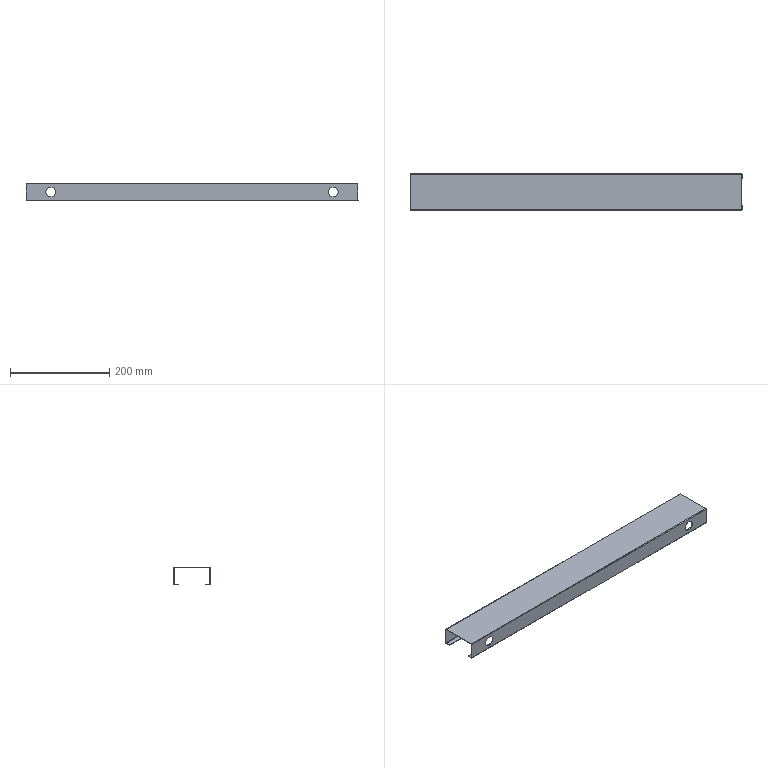Part | SolidWorks | features EdgeFlange 2, Cut 1, FlatPattern 1, ICE 1, SMBaseFlange 1, SheetMetal 1 | 1 solid | 46 faces | box 668 x 74 x 35 mm | volume 104821 mm3 | plane 30 | cylinder 16 | commonest cylinder face diameters 20 x8 0.4 x4 2.4 x4
STEP:
#1=CARTESIAN_POINT('',(-284.,36.,-27.5));
#2=VERTEX_POINT('',#1);
#3=CARTESIAN_POINT('',(-284.,36.,-7.5));
#4=VERTEX_POINT('',#3);
#5=CARTESIAN_POINT('',(-284.,36.,-17.5));
#6=DIRECTION('',(0.,1.,0.));
#7=DIRECTION('',(0.,0.,1.));
#8=AXIS2_PLACEMENT_3D('',#5,#6,#7);
#9=CIRCLE('',#8,10.);
#10=EDGE_CURVE('',#2,#4,#9,.T.);
#11=ORIENTED_EDGE('',*,*,#10,.F.);
#12=CARTESIAN_POINT('',(-284.,37.,-27.5));
#13=VERTEX_POINT('',#12);
#14=CARTESIAN_POINT('',(-284.,-37.,-27.5));
#15=DIRECTION('',(0.,1.,0.));
#16=VECTOR('',#15,1000.);
#17=LINE('',#14,#16);
#18=EDGE_CURVE('',#2,#13,#17,.T.);
#19=ORIENTED_EDGE('',*,*,#18,.T.);
#20=CARTESIAN_POINT('',(-284.,37.,-7.5));
#21=VERTEX_POINT('',#20);
#22=CARTESIAN_POINT('',(-284.,37.,-17.5));
#23=DIRECTION('',(0.,1.,0.));
#24=DIRECTION('',(0.,0.,1.));
#25=AXIS2_PLACEMENT_3D('',#22,#23,#24);
#26=CIRCLE('',#25,10.);
#27=EDGE_CURVE('',#13,#21,#26,.T.);
#28=ORIENTED_EDGE('',*,*,#27,.T.);
#29=CARTESIAN_POINT('',(-284.,-37.,-7.5));
#30=DIRECTION('',(0.,1.,0.));
#31=VECTOR('',#30,1000.);
#32=LINE('',#29,#31);
#33=EDGE_CURVE('',#4,#21,#32,.T.);
#34=ORIENTED_EDGE('',*,*,#33,.F.);
#35=EDGE_LOOP('',(#11,#19,#28,#34));
#36=FACE_OUTER_BOUND('',#35,.T.);
#37=CARTESIAN_POINT('',(-284.,-37.,-17.5));
#38=DIRECTION('',(0.,1.,0.));
#39=DIRECTION('',(0.,0.,1.));
#40=AXIS2_PLACEMENT_3D('',#37,#38,#39);
#41=CYLINDRICAL_SURFACE('',#40,10.);
#42=ADVANCED_FACE('',(#36),#41,.F.);
#43=CARTESIAN_POINT('',(284.,36.,-27.5));
#44=VERTEX_POINT('',#43);
#45=CARTESIAN_POINT('',(284.,36.,-7.5));
#46=VERTEX_POINT('',#45);
#47=CARTESIAN_POINT('',(284.,36.,-17.5));
#48=DIRECTION('',(0.,1.,0.));
#49=DIRECTION('',(0.,0.,1.));
#50=AXIS2_PLACEMENT_3D('',#47,#48,#49);
#51=CIRCLE('',#50,10.);
#52=EDGE_CURVE('',#44,#46,#51,.T.);
#53=ORIENTED_EDGE('',*,*,#52,.F.);
#54=CARTESIAN_POINT('',(284.,37.,-27.5));
#55=VERTEX_POINT('',#54);
#56=CARTESIAN_POINT('',(284.,-37.,-27.5));
#57=DIRECTION('',(0.,1.,0.));
#58=VECTOR('',#57,1000.);
#59=LINE('',#56,#58);
#60=EDGE_CURVE('',#44,#55,#59,.T.);
#61=ORIENTED_EDGE('',*,*,#60,.T.);
#62=CARTESIAN_POINT('',(284.,37.,-7.5));
#63=VERTEX_POINT('',#62);
#64=CARTESIAN_POINT('',(284.,37.,-17.5));
#65=DIRECTION('',(0.,1.,0.));
#66=DIRECTION('',(0.,0.,1.));
#67=AXIS2_PLACEMENT_3D('',#64,#65,#66);
#68=CIRCLE('',#67,10.);
#69=EDGE_CURVE('',#55,#63,#68,.T.);
#70=ORIENTED_EDGE('',*,*,#69,.T.);
#71=CARTESIAN_POINT('',(284.,-37.,-7.5));
#72=DIRECTION('',(0.,1.,0.));
#73=VECTOR('',#72,1000.);
#74=LINE('',#71,#73);
#75=EDGE_CURVE('',#46,#63,#74,.T.);
#76=ORIENTED_EDGE('',*,*,#75,.F.);
#77=EDGE_LOOP('',(#53,#61,#70,#76));
#78=FACE_OUTER_BOUND('',#77,.T.);
#79=CARTESIAN_POINT('',(284.,-37.,-17.5));
#80=DIRECTION('',(0.,1.,0.));
#81=DIRECTION('',(0.,0.,1.));
#82=AXIS2_PLACEMENT_3D('',#79,#80,#81);
#83=CYLINDRICAL_SURFACE('',#82,10.);
#84=ADVANCED_FACE('',(#78),#83,.F.);
#85=CARTESIAN_POINT('',(-284.,-37.,-27.5));
#86=VERTEX_POINT('',#85);
#87=CARTESIAN_POINT('',(-284.,-37.,-7.5));
#88=VERTEX_POINT('',#87);
#89=CARTESIAN_POINT('',(-284.,-37.,-17.5));
#90=DIRECTION('',(0.,1.,0.));
#91=DIRECTION('',(0.,0.,1.));
#92=AXIS2_PLACEMENT_3D('',#89,#90,#91);
#93=CIRCLE('',#92,10.);
#94=EDGE_CURVE('',#86,#88,#93,.T.);
#95=ORIENTED_EDGE('',*,*,#94,.F.);
#96=CARTESIAN_POINT('',(-284.,-36.,-27.5));
#97=VERTEX_POINT('',#96);
#98=CARTESIAN_POINT('',(-284.,-37.,-27.5));
#99=DIRECTION('',(0.,1.,0.));
#100=VECTOR('',#99,1000.);
#101=LINE('',#98,#100);
#102=EDGE_CURVE('',#86,#97,#101,.T.);
#103=ORIENTED_EDGE('',*,*,#102,.T.);
#104=CARTESIAN_POINT('',(-284.,-36.,-7.5));
#105=VERTEX_POINT('',#104);
#106=CARTESIAN_POINT('',(-284.,-36.,-17.5));
#107=DIRECTION('',(0.,1.,0.));
#108=DIRECTION('',(0.,0.,1.));
#109=AXIS2_PLACEMENT_3D('',#106,#107,#108);
#110=CIRCLE('',#109,10.);
#111=EDGE_CURVE('',#97,#105,#110,.T.);
#112=ORIENTED_EDGE('',*,*,#111,.T.);
#113=CARTESIAN_POINT('',(-284.,-37.,-7.5));
#114=DIRECTION('',(0.,1.,0.));
#115=VECTOR('',#114,1000.);
#116=LINE('',#113,#115);
#117=EDGE_CURVE('',#88,#105,#116,.T.);
#118=ORIENTED_EDGE('',*,*,#117,.F.);
#119=EDGE_LOOP('',(#95,#103,#112,#118));
#120=FACE_OUTER_BOUND('',#119,.T.);
#121=CARTESIAN_POINT('',(-284.,-37.,-17.5));
#122=DIRECTION('',(0.,1.,0.));
#123=DIRECTION('',(0.,0.,1.));
#124=AXIS2_PLACEMENT_3D('',#121,#122,#123);
#125=CYLINDRICAL_SURFACE('',#124,10.);
#126=ADVANCED_FACE('',(#120),#125,.F.);
#127=CARTESIAN_POINT('',(284.,-37.,-27.5));
#128=VERTEX_POINT('',#127);
#129=CARTESIAN_POINT('',(284.,-37.,-7.5));
#130=VERTEX_POINT('',#129);
#131=CARTESIAN_POINT('',(284.,-37.,-17.5));
#132=DIRECTION('',(0.,1.,0.));
#133=DIRECTION('',(0.,0.,-1.));
#134=AXIS2_PLACEMENT_3D('',#131,#132,#133);
#135=CIRCLE('',#134,10.);
#136=EDGE_CURVE('',#128,#130,#135,.T.);
#137=ORIENTED_EDGE('',*,*,#136,.F.);
#138=CARTESIAN_POINT('',(284.,-36.,-27.5));
#139=VERTEX_POINT('',#138);
#140=CARTESIAN_POINT('',(284.,-37.,-27.5));
#141=DIRECTION('',(0.,1.,0.));
#142=VECTOR('',#141,1000.);
#143=LINE('',#140,#142);
#144=EDGE_CURVE('',#128,#139,#143,.T.);
#145=ORIENTED_EDGE('',*,*,#144,.T.);
#146=CARTESIAN_POINT('',(284.,-36.,-7.5));
#147=VERTEX_POINT('',#146);
#148=CARTESIAN_POINT('',(284.,-36.,-17.5));
#149=DIRECTION('',(0.,1.,0.));
#150=DIRECTION('',(0.,0.,1.));
#151=AXIS2_PLACEMENT_3D('',#148,#149,#150);
#152=CIRCLE('',#151,10.);
#153=EDGE_CURVE('',#139,#147,#152,.T.);
#154=ORIENTED_EDGE('',*,*,#153,.T.);
#155=CARTESIAN_POINT('',(284.,-37.,-7.5));
#156=DIRECTION('',(0.,1.,0.));
#157=VECTOR('',#156,1000.);
#158=LINE('',#155,#157);
#159=EDGE_CURVE('',#130,#147,#158,.T.);
#160=ORIENTED_EDGE('',*,*,#159,.F.);
#161=EDGE_LOOP('',(#137,#145,#154,#160));
#162=FACE_OUTER_BOUND('',#161,.T.);
#163=CARTESIAN_POINT('',(284.,-37.,-17.5));
#164=DIRECTION('',(0.,1.,0.));
#165=DIRECTION('',(0.,0.,1.));
#166=AXIS2_PLACEMENT_3D('',#163,#164,#165);
#167=CYLINDRICAL_SURFACE('',#166,10.);
#168=ADVANCED_FACE('',(#162),#167,.F.);
#169=CARTESIAN_POINT('',(334.,36.,-33.8));
#170=VERTEX_POINT('',#169);
#171=CARTESIAN_POINT('',(334.,36.,-1.2));
#172=VERTEX_POINT('',#171);
#173=CARTESIAN_POINT('',(334.,36.,0.));
#174=DIRECTION('',(0.,0.,1.));
#175=VECTOR('',#174,1000.);
#176=LINE('',#173,#175);
#177=EDGE_CURVE('',#170,#172,#176,.T.);
#178=ORIENTED_EDGE('',*,*,#177,.F.);
#179=CARTESIAN_POINT('',(334.,37.,-33.8));
#180=VERTEX_POINT('',#179);
#181=CARTESIAN_POINT('',(334.,36.,-33.8));
#182=DIRECTION('',(0.,1.,0.));
#183=VECTOR('',#182,1000.);
#184=LINE('',#181,#183);
#185=EDGE_CURVE('',#170,#180,#184,.T.);
#186=ORIENTED_EDGE('',*,*,#185,.T.);
#187=CARTESIAN_POINT('',(334.,37.,-1.2));
#188=VERTEX_POINT('',#187);
#189=CARTESIAN_POINT('',(334.,37.,-1.));
#190=DIRECTION('',(0.,0.,1.));
#191=VECTOR('',#190,1000.);
#192=LINE('',#189,#191);
#193=EDGE_CURVE('',#180,#188,#192,.T.);
#194=ORIENTED_EDGE('',*,*,#193,.T.);
#195=CARTESIAN_POINT('',(334.,36.,-1.2));
#196=DIRECTION('',(0.,1.,0.));
#197=VECTOR('',#196,1000.);
#198=LINE('',#195,#197);
#199=EDGE_CURVE('',#172,#188,#198,.T.);
#200=ORIENTED_EDGE('',*,*,#199,.F.);
#201=EDGE_LOOP('',(#178,#186,#194,#200));
#202=FACE_OUTER_BOUND('',#201,.T.);
#203=CARTESIAN_POINT('',(334.,37.,-1.));
#204=DIRECTION('',(1.,0.,0.));
#205=DIRECTION('',(0.,0.,-1.));
#206=AXIS2_PLACEMENT_3D('',#203,#204,#205);
#207=PLANE('',#206);
#208=ADVANCED_FACE('',(#202),#207,.T.);
#209=CARTESIAN_POINT('',(-284.,37.,-17.5));
#210=DIRECTION('',(0.,1.,0.));
#211=DIRECTION('',(0.,0.,1.));
#212=AXIS2_PLACEMENT_3D('',#209,#210,#211);
#213=CIRCLE('',#212,10.);
#214=EDGE_CURVE('',#21,#13,#213,.T.);
#215=ORIENTED_EDGE('',*,*,#214,.F.);
#216=ORIENTED_EDGE('',*,*,#27,.F.);
#217=EDGE_LOOP('',(#215,#216));
#218=FACE_BOUND('',#217,.T.);
#219=CARTESIAN_POINT('',(284.,37.,-17.5));
#220=DIRECTION('',(0.,1.,0.));
#221=DIRECTION('',(0.,0.,1.));
#222=AXIS2_PLACEMENT_3D('',#219,#220,#221);
#223=CIRCLE('',#222,10.);
#224=EDGE_CURVE('',#63,#55,#223,.T.);
#225=ORIENTED_EDGE('',*,*,#224,.F.);
#226=ORIENTED_EDGE('',*,*,#69,.F.);
#227=EDGE_LOOP('',(#225,#226));
#228=FACE_BOUND('',#227,.T.);
#229=ORIENTED_EDGE('',*,*,#193,.F.);
#230=CARTESIAN_POINT('',(-334.,37.,-33.8));
#231=VERTEX_POINT('',#230);
#232=CARTESIAN_POINT('',(334.,37.,-33.8));
#233=DIRECTION('',(-1.,0.,0.));
#234=VECTOR('',#233,1000.);
#235=LINE('',#232,#234);
#236=EDGE_CURVE('',#180,#231,#235,.T.);
#237=ORIENTED_EDGE('',*,*,#236,.T.);
#238=CARTESIAN_POINT('',(-334.,37.,-1.2));
#239=VERTEX_POINT('',#238);
#240=CARTESIAN_POINT('',(-334.,37.,-35.));
#241=DIRECTION('',(0.,0.,-1.));
#242=VECTOR('',#241,1000.);
#243=LINE('',#240,#242);
#244=EDGE_CURVE('',#239,#231,#243,.T.);
#245=ORIENTED_EDGE('',*,*,#244,.F.);
#246=CARTESIAN_POINT('',(0.,37.,-1.2));
#247=DIRECTION('',(1.,0.,0.));
#248=VECTOR('',#247,1000.);
#249=LINE('',#246,#248);
#250=EDGE_CURVE('',#239,#188,#249,.T.);
#251=ORIENTED_EDGE('',*,*,#250,.T.);
#252=EDGE_LOOP('',(#229,#237,#245,#251));
#253=FACE_OUTER_BOUND('',#252,.T.);
#254=CARTESIAN_POINT('',(0.,37.,0.));
#255=DIRECTION('',(0.,1.,0.));
#256=DIRECTION('',(0.,0.,1.));
#257=AXIS2_PLACEMENT_3D('',#254,#255,#256);
#258=PLANE('',#257);
#259=ADVANCED_FACE('',(#218,#228,#253),#258,.T.);
#260=CARTESIAN_POINT('',(-284.,36.,-17.5));
#261=DIRECTION('',(0.,1.,0.));
#262=DIRECTION('',(0.,0.,1.));
#263=AXIS2_PLACEMENT_3D('',#260,#261,#262);
#264=CIRCLE('',#263,10.);
#265=EDGE_CURVE('',#4,#2,#264,.T.);
#266=ORIENTED_EDGE('',*,*,#265,.T.);
#267=ORIENTED_EDGE('',*,*,#10,.T.);
#268=EDGE_LOOP('',(#266,#267));
#269=FACE_BOUND('',#268,.T.);
#270=CARTESIAN_POINT('',(284.,36.,-17.5));
#271=DIRECTION('',(0.,1.,0.));
#272=DIRECTION('',(0.,0.,1.));
#273=AXIS2_PLACEMENT_3D('',#270,#271,#272);
#274=CIRCLE('',#273,10.);
#275=EDGE_CURVE('',#46,#44,#274,.T.);
#276=ORIENTED_EDGE('',*,*,#275,.T.);
#277=ORIENTED_EDGE('',*,*,#52,.T.);
#278=EDGE_LOOP('',(#276,#277));
#279=FACE_BOUND('',#278,.T.);
#280=CARTESIAN_POINT('',(-334.,36.,-33.8));
#281=VERTEX_POINT('',#280);
#282=CARTESIAN_POINT('',(334.,36.,-33.8));
#283=DIRECTION('',(-1.,0.,0.));
#284=VECTOR('',#283,1000.);
#285=LINE('',#282,#284);
#286=EDGE_CURVE('',#170,#281,#285,.T.);
#287=ORIENTED_EDGE('',*,*,#286,.F.);
#288=ORIENTED_EDGE('',*,*,#177,.T.);
#289=CARTESIAN_POINT('',(-334.,36.,-1.2));
#290=VERTEX_POINT('',#289);
#291=CARTESIAN_POINT('',(-334.,36.,-1.2));
#292=DIRECTION('',(1.,0.,0.));
#293=VECTOR('',#292,1000.);
#294=LINE('',#291,#293);
#295=EDGE_CURVE('',#290,#172,#294,.T.);
#296=ORIENTED_EDGE('',*,*,#295,.F.);
#297=CARTESIAN_POINT('',(-334.,36.,0.));
#298=DIRECTION('',(0.,0.,-1.));
#299=VECTOR('',#298,1000.);
#300=LINE('',#297,#299);
#301=EDGE_CURVE('',#290,#281,#300,.T.);
#302=ORIENTED_EDGE('',*,*,#301,.T.);
#303=EDGE_LOOP('',(#287,#288,#296,#302));
#304=FACE_OUTER_BOUND('',#303,.T.);
#305=CARTESIAN_POINT('',(0.,36.,0.));
#306=DIRECTION('',(0.,1.,0.));
#307=DIRECTION('',(0.,0.,1.));
#308=AXIS2_PLACEMENT_3D('',#305,#306,#307);
#309=PLANE('',#308);
#310=ADVANCED_FACE('',(#269,#279,#304),#309,.F.);
#311=CARTESIAN_POINT('',(-334.,-36.,-33.8));
#312=VERTEX_POINT('',#311);
#313=CARTESIAN_POINT('',(-334.,-36.,-1.2));
#314=VERTEX_POINT('',#313);
#315=CARTESIAN_POINT('',(-334.,-36.,0.));
#316=DIRECTION('',(0.,0.,1.));
#317=VECTOR('',#316,1000.);
#318=LINE('',#315,#317);
#319=EDGE_CURVE('',#312,#314,#318,.T.);
#320=ORIENTED_EDGE('',*,*,#319,.F.);
#321=CARTESIAN_POINT('',(-334.,-37.,-33.8));
#322=VERTEX_POINT('',#321);
#323=CARTESIAN_POINT('',(-334.,-36.,-33.8));
#324=DIRECTION('',(0.,-1.,0.));
#325=VECTOR('',#324,1000.);
#326=LINE('',#323,#325);
#327=EDGE_CURVE('',#312,#322,#326,.T.);
#328=ORIENTED_EDGE('',*,*,#327,.T.);
#329=CARTESIAN_POINT('',(-334.,-37.,-1.2));
#330=VERTEX_POINT('',#329);
#331=CARTESIAN_POINT('',(-334.,-37.,-35.));
#332=DIRECTION('',(0.,0.,1.));
#333=VECTOR('',#332,1000.);
#334=LINE('',#331,#333);
#335=EDGE_CURVE('',#322,#330,#334,.T.);
#336=ORIENTED_EDGE('',*,*,#335,.T.);
#337=CARTESIAN_POINT('',(-334.,-36.,-1.2));
#338=DIRECTION('',(0.,-1.,0.));
#339=VECTOR('',#338,1000.);
#340=LINE('',#337,#339);
#341=EDGE_CURVE('',#314,#330,#340,.T.);
#342=ORIENTED_EDGE('',*,*,#341,.F.);
#343=EDGE_LOOP('',(#320,#328,#336,#342));
#344=FACE_OUTER_BOUND('',#343,.T.);
#345=CARTESIAN_POINT('',(-334.,-37.,-35.));
#346=DIRECTION('',(-1.,0.,0.));
#347=DIRECTION('',(0.,0.,1.));
#348=AXIS2_PLACEMENT_3D('',#345,#346,#347);
#349=PLANE('',#348);
#350=ADVANCED_FACE('',(#344),#349,.T.);
#351=CARTESIAN_POINT('',(-284.,-37.,-17.5));
#352=DIRECTION('',(0.,1.,0.));
#353=DIRECTION('',(0.,0.,1.));
#354=AXIS2_PLACEMENT_3D('',#351,#352,#353);
#355=CIRCLE('',#354,10.);
#356=EDGE_CURVE('',#88,#86,#355,.T.);
#357=ORIENTED_EDGE('',*,*,#356,.T.);
#358=ORIENTED_EDGE('',*,*,#94,.T.);
#359=EDGE_LOOP('',(#357,#358));
#360=FACE_BOUND('',#359,.T.);
#361=CARTESIAN_POINT('',(284.,-37.,-17.5));
#362=DIRECTION('',(0.,1.,0.));
#363=DIRECTION('',(0.,0.,-1.));
#364=AXIS2_PLACEMENT_3D('',#361,#362,#363);
#365=CIRCLE('',#364,10.);
#366=EDGE_CURVE('',#130,#128,#365,.T.);
#367=ORIENTED_EDGE('',*,*,#366,.T.);
#368=ORIENTED_EDGE('',*,*,#136,.T.);
#369=EDGE_LOOP('',(#367,#368));
#370=FACE_BOUND('',#369,.T.);
#371=CARTESIAN_POINT('',(334.,-37.,-33.8));
#372=VERTEX_POINT('',#371);
#373=CARTESIAN_POINT('',(-334.,-37.,-33.8));
#374=DIRECTION('',(1.,0.,0.));
#375=VECTOR('',#374,1000.);
#376=LINE('',#373,#375);
#377=EDGE_CURVE('',#322,#372,#376,.T.);
#378=ORIENTED_EDGE('',*,*,#377,.T.);
#379=CARTESIAN_POINT('',(334.,-37.,-1.2));
#380=VERTEX_POINT('',#379);
#381=CARTESIAN_POINT('',(334.,-37.,-1.));
#382=DIRECTION('',(0.,0.,-1.));
#383=VECTOR('',#382,1000.);
#384=LINE('',#381,#383);
#385=EDGE_CURVE('',#380,#372,#384,.T.);
#386=ORIENTED_EDGE('',*,*,#385,.F.);
#387=CARTESIAN_POINT('',(334.,-37.,-1.2));
#388=DIRECTION('',(1.,0.,0.));
#389=VECTOR('',#388,1000.);
#390=LINE('',#387,#389);
#391=EDGE_CURVE('',#330,#380,#390,.T.);
#392=ORIENTED_EDGE('',*,*,#391,.F.);
#393=ORIENTED_EDGE('',*,*,#335,.F.);
#394=EDGE_LOOP('',(#378,#386,#392,#393));
#395=FACE_OUTER_BOUND('',#394,.T.);
#396=CARTESIAN_POINT('',(0.,-37.,0.));
#397=DIRECTION('',(0.,1.,0.));
#398=DIRECTION('',(0.,0.,1.));
#399=AXIS2_PLACEMENT_3D('',#396,#397,#398);
#400=PLANE('',#399);
#401=ADVANCED_FACE('',(#360,#370,#395),#400,.F.);
#402=CARTESIAN_POINT('',(-284.,-36.,-17.5));
#403=DIRECTION('',(0.,1.,0.));
#404=DIRECTION('',(0.,0.,1.));
#405=AXIS2_PLACEMENT_3D('',#402,#403,#404);
#406=CIRCLE('',#405,10.);
#407=EDGE_CURVE('',#105,#97,#406,.T.);
#408=ORIENTED_EDGE('',*,*,#407,.F.);
#409=ORIENTED_EDGE('',*,*,#111,.F.);
#410=EDGE_LOOP('',(#408,#409));
#411=FACE_BOUND('',#410,.T.);
#412=CARTESIAN_POINT('',(284.,-36.,-17.5));
#413=DIRECTION('',(0.,1.,0.));
#414=DIRECTION('',(0.,0.,1.));
#415=AXIS2_PLACEMENT_3D('',#412,#413,#414);
#416=CIRCLE('',#415,10.);
#417=EDGE_CURVE('',#147,#139,#416,.T.);
#418=ORIENTED_EDGE('',*,*,#417,.F.);
#419=ORIENTED_EDGE('',*,*,#153,.F.);
#420=EDGE_LOOP('',(#418,#419));
#421=FACE_BOUND('',#420,.T.);
#422=CARTESIAN_POINT('',(334.,-36.,-1.2));
#423=VERTEX_POINT('',#422);
#424=CARTESIAN_POINT('',(334.,-36.,-33.8));
#425=VERTEX_POINT('',#424);
#426=CARTESIAN_POINT('',(334.,-36.,0.));
#427=DIRECTION('',(0.,0.,-1.));
#428=VECTOR('',#427,1000.);
#429=LINE('',#426,#428);
#430=EDGE_CURVE('',#423,#425,#429,.T.);
#431=ORIENTED_EDGE('',*,*,#430,.T.);
#432=CARTESIAN_POINT('',(-334.,-36.,-33.8));
#433=DIRECTION('',(1.,0.,0.));
#434=VECTOR('',#433,1000.);
#435=LINE('',#432,#434);
#436=EDGE_CURVE('',#312,#425,#435,.T.);
#437=ORIENTED_EDGE('',*,*,#436,.F.);
#438=ORIENTED_EDGE('',*,*,#319,.T.);
#439=CARTESIAN_POINT('',(334.,-36.,-1.2));
#440=DIRECTION('',(-1.,0.,0.));
#441=VECTOR('',#440,1000.);
#442=LINE('',#439,#441);
#443=EDGE_CURVE('',#423,#314,#442,.T.);
#444=ORIENTED_EDGE('',*,*,#443,.F.);
#445=EDGE_LOOP('',(#431,#437,#438,#444));
#446=FACE_OUTER_BOUND('',#445,.T.);
#447=CARTESIAN_POINT('',(0.,-36.,0.));
#448=DIRECTION('',(0.,1.,0.));
#449=DIRECTION('',(0.,0.,1.));
#450=AXIS2_PLACEMENT_3D('',#447,#448,#449);
#451=PLANE('',#450);
#452=ADVANCED_FACE('',(#411,#421,#446),#451,.T.);
#453=CARTESIAN_POINT('',(-334.,-35.8,-1.));
#454=VERTEX_POINT('',#453);
#455=CARTESIAN_POINT('',(334.,-35.8,-1.));
#456=VERTEX_POINT('',#455);
#457=CARTESIAN_POINT('',(-334.,-35.8,-1.));
#458=DIRECTION('',(1.,0.,0.));
#459=VECTOR('',#458,1000.);
#460=LINE('',#457,#459);
#461=EDGE_CURVE('',#454,#456,#460,.T.);
#462=ORIENTED_EDGE('',*,*,#461,.F.);
#463=CARTESIAN_POINT('',(-334.,35.8,-1.));
#464=VERTEX_POINT('',#463);
#465=CARTESIAN_POINT('',(-334.,37.,-1.));
#466=DIRECTION('',(0.,-1.,0.));
#467=VECTOR('',#466,1000.);
#468=LINE('',#465,#467);
#469=EDGE_CURVE('',#464,#454,#468,.T.);
#470=ORIENTED_EDGE('',*,*,#469,.F.);
#471=CARTESIAN_POINT('',(334.,35.8,-1.));
#472=VERTEX_POINT('',#471);
#473=CARTESIAN_POINT('',(334.,35.8,-1.));
#474=DIRECTION('',(-1.,0.,0.));
#475=VECTOR('',#474,1000.);
#476=LINE('',#473,#475);
#477=EDGE_CURVE('',#472,#464,#476,.T.);
#478=ORIENTED_EDGE('',*,*,#477,.F.);
#479=CARTESIAN_POINT('',(334.,37.,-1.));
#480=DIRECTION('',(0.,1.,0.));
#481=VECTOR('',#480,1000.);
#482=LINE('',#479,#481);
#483=EDGE_CURVE('',#456,#472,#482,.T.);
#484=ORIENTED_EDGE('',*,*,#483,.F.);
#485=EDGE_LOOP('',(#462,#470,#478,#484));
#486=FACE_OUTER_BOUND('',#485,.T.);
#487=CARTESIAN_POINT('',(0.,0.,-1.));
#488=DIRECTION('',(0.,0.,1.));
#489=DIRECTION('',(1.,0.,0.));
#490=AXIS2_PLACEMENT_3D('',#487,#488,#489);
#491=PLANE('',#490);
#492=ADVANCED_FACE('',(#486),#491,.F.);
#493=CARTESIAN_POINT('',(-334.,35.8,0.));
#494=VERTEX_POINT('',#493);
#495=CARTESIAN_POINT('',(-334.,-35.8,0.));
#496=VERTEX_POINT('',#495);
#497=CARTESIAN_POINT('',(-334.,37.,0.));
#498=DIRECTION('',(0.,-1.,0.));
#499=VECTOR('',#498,1000.);
#500=LINE('',#497,#499);
#501=EDGE_CURVE('',#494,#496,#500,.T.);
#502=ORIENTED_EDGE('',*,*,#501,.T.);
#503=CARTESIAN_POINT('',(334.,-35.8,0.));
#504=VERTEX_POINT('',#503);
#505=CARTESIAN_POINT('',(-334.,-35.8,0.));
#506=DIRECTION('',(1.,0.,0.));
#507=VECTOR('',#506,1000.);
#508=LINE('',#505,#507);
#509=EDGE_CURVE('',#496,#504,#508,.T.);
#510=ORIENTED_EDGE('',*,*,#509,.T.);
#511=CARTESIAN_POINT('',(334.,35.8,0.));
#512=VERTEX_POINT('',#511);
#513=CARTESIAN_POINT('',(334.,37.,0.));
#514=DIRECTION('',(0.,1.,0.));
#515=VECTOR('',#514,1000.);
#516=LINE('',#513,#515);
#517=EDGE_CURVE('',#504,#512,#516,.T.);
#518=ORIENTED_EDGE('',*,*,#517,.T.);
#519=CARTESIAN_POINT('',(334.,35.8,0.));
#520=DIRECTION('',(-1.,0.,0.));
#521=VECTOR('',#520,1000.);
#522=LINE('',#519,#521);
#523=EDGE_CURVE('',#512,#494,#522,.T.);
#524=ORIENTED_EDGE('',*,*,#523,.T.);
#525=EDGE_LOOP('',(#502,#510,#518,#524));
#526=FACE_OUTER_BOUND('',#525,.T.);
#527=CARTESIAN_POINT('',(0.,0.,0.));
#528=DIRECTION('',(0.,0.,1.));
#529=DIRECTION('',(1.,0.,0.));
#530=AXIS2_PLACEMENT_3D('',#527,#528,#529);
#531=PLANE('',#530);
#532=ADVANCED_FACE('',(#526),#531,.T.);
#533=ORIENTED_EDGE('',*,*,#469,.T.);
#534=CARTESIAN_POINT('',(-334.,-35.8,-1.));
#535=DIRECTION('',(0.,0.,1.));
#536=VECTOR('',#535,1000.);
#537=LINE('',#534,#536);
#538=EDGE_CURVE('',#454,#496,#537,.T.);
#539=ORIENTED_EDGE('',*,*,#538,.T.);
#540=ORIENTED_EDGE('',*,*,#501,.F.);
#541=CARTESIAN_POINT('',(-334.,35.8,-1.));
#542=DIRECTION('',(0.,0.,1.));
#543=VECTOR('',#542,1000.);
#544=LINE('',#541,#543);
#545=EDGE_CURVE('',#464,#494,#544,.T.);
#546=ORIENTED_EDGE('',*,*,#545,.F.);
#547=EDGE_LOOP('',(#533,#539,#540,#546));
#548=FACE_OUTER_BOUND('',#547,.T.);
#549=CARTESIAN_POINT('',(-334.,37.,-1.));
#550=DIRECTION('',(-1.,0.,0.));
#551=DIRECTION('',(0.,0.,1.));
#552=AXIS2_PLACEMENT_3D('',#549,#550,#551);
#553=PLANE('',#552);
#554=ADVANCED_FACE('',(#548),#553,.T.);
#555=CARTESIAN_POINT('',(334.,-35.8,-1.));
#556=DIRECTION('',(0.,0.,1.));
#557=VECTOR('',#556,1000.);
#558=LINE('',#555,#557);
#559=EDGE_CURVE('',#456,#504,#558,.T.);
#560=ORIENTED_EDGE('',*,*,#559,.F.);
#561=ORIENTED_EDGE('',*,*,#483,.T.);
#562=CARTESIAN_POINT('',(334.,35.8,-1.));
#563=DIRECTION('',(0.,0.,1.));
#564=VECTOR('',#563,1000.);
#565=LINE('',#562,#564);
#566=EDGE_CURVE('',#472,#512,#565,.T.);
#567=ORIENTED_EDGE('',*,*,#566,.T.);
#568=ORIENTED_EDGE('',*,*,#517,.F.);
#569=EDGE_LOOP('',(#560,#561,#567,#568));
#570=FACE_OUTER_BOUND('',#569,.T.);
#571=CARTESIAN_POINT('',(334.,37.,-1.));
#572=DIRECTION('',(1.,0.,0.));
#573=DIRECTION('',(0.,0.,-1.));
#574=AXIS2_PLACEMENT_3D('',#571,#572,#573);
#575=PLANE('',#574);
#576=ADVANCED_FACE('',(#570),#575,.T.);
#577=CARTESIAN_POINT('',(-334.,37.,-1.2));
#578=DIRECTION('',(0.,1.,0.));
#579=VECTOR('',#578,1000.);
#580=LINE('',#577,#579);
#581=EDGE_CURVE('',#290,#239,#580,.T.);
#582=ORIENTED_EDGE('',*,*,#581,.F.);
#583=CARTESIAN_POINT('',(-334.,35.8,-1.2));
#584=DIRECTION('',(-1.,0.,0.));
#585=DIRECTION('',(0.,0.,-1.));
#586=AXIS2_PLACEMENT_3D('',#583,#584,#585);
#587=CIRCLE('',#586,0.2);
#588=EDGE_CURVE('',#464,#290,#587,.T.);
#589=ORIENTED_EDGE('',*,*,#588,.F.);
#590=ORIENTED_EDGE('',*,*,#545,.T.);
#591=CARTESIAN_POINT('',(-334.,35.8,-1.2));
#592=DIRECTION('',(-1.,0.,0.));
#593=DIRECTION('',(0.,0.,-1.));
#594=AXIS2_PLACEMENT_3D('',#591,#592,#593);
#595=CIRCLE('',#594,1.2);
#596=EDGE_CURVE('',#494,#239,#595,.T.);
#597=ORIENTED_EDGE('',*,*,#596,.T.);
#598=EDGE_LOOP('',(#582,#589,#590,#597));
#599=FACE_OUTER_BOUND('',#598,.T.);
#600=CARTESIAN_POINT('',(-334.,35.8,-1.2));
#601=DIRECTION('',(-1.,0.,0.));
#602=DIRECTION('',(0.,0.,1.));
#603=AXIS2_PLACEMENT_3D('',#600,#601,#602);
#604=PLANE('',#603);
#605=ADVANCED_FACE('',(#599),#604,.T.);
#606=CARTESIAN_POINT('',(334.,35.8,-1.2));
#607=DIRECTION('',(1.,0.,0.));
#608=DIRECTION('',(0.,0.,-1.));
#609=AXIS2_PLACEMENT_3D('',#606,#607,#608);
#610=CIRCLE('',#609,0.2);
#611=EDGE_CURVE('',#172,#472,#610,.T.);
#612=ORIENTED_EDGE('',*,*,#611,.F.);
#613=ORIENTED_EDGE('',*,*,#199,.T.);
#614=CARTESIAN_POINT('',(334.,35.8,-1.2));
#615=DIRECTION('',(1.,0.,0.));
#616=DIRECTION('',(0.,0.,-1.));
#617=AXIS2_PLACEMENT_3D('',#614,#615,#616);
#618=CIRCLE('',#617,1.2);
#619=EDGE_CURVE('',#188,#512,#618,.T.);
#620=ORIENTED_EDGE('',*,*,#619,.T.);
#621=ORIENTED_EDGE('',*,*,#566,.F.);
#622=EDGE_LOOP('',(#612,#613,#620,#621));
#623=FACE_OUTER_BOUND('',#622,.T.);
#624=CARTESIAN_POINT('',(334.,35.8,-1.2));
#625=DIRECTION('',(-1.,0.,0.));
#626=DIRECTION('',(0.,0.,1.));
#627=AXIS2_PLACEMENT_3D('',#624,#625,#626);
#628=PLANE('',#627);
#629=ADVANCED_FACE('',(#623),#628,.F.);
#630=ORIENTED_EDGE('',*,*,#523,.F.);
#631=ORIENTED_EDGE('',*,*,#619,.F.);
#632=ORIENTED_EDGE('',*,*,#250,.F.);
#633=ORIENTED_EDGE('',*,*,#596,.F.);
#634=EDGE_LOOP('',(#630,#631,#632,#633));
#635=FACE_OUTER_BOUND('',#634,.T.);
#636=CARTESIAN_POINT('',(334.,35.8,-1.2));
#637=DIRECTION('',(1.,0.,0.));
#638=DIRECTION('',(0.,1.,0.));
#639=AXIS2_PLACEMENT_3D('',#636,#637,#638);
#640=CYLINDRICAL_SURFACE('',#639,1.2);
#641=ADVANCED_FACE('',(#635),#640,.T.);
#642=ORIENTED_EDGE('',*,*,#477,.T.);
#643=ORIENTED_EDGE('',*,*,#588,.T.);
#644=ORIENTED_EDGE('',*,*,#295,.T.);
#645=ORIENTED_EDGE('',*,*,#611,.T.);
#646=EDGE_LOOP('',(#642,#643,#644,#645));
#647=FACE_OUTER_BOUND('',#646,.T.);
#648=CARTESIAN_POINT('',(334.,35.8,-1.2));
#649=DIRECTION('',(1.,0.,0.));
#650=DIRECTION('',(0.,1.,0.));
#651=AXIS2_PLACEMENT_3D('',#648,#649,#650);
#652=CYLINDRICAL_SURFACE('',#651,0.2);
#653=ADVANCED_FACE('',(#647),#652,.F.);
#654=CARTESIAN_POINT('',(-334.,36.,-33.8));
#655=DIRECTION('',(0.,1.,0.));
#656=VECTOR('',#655,1000.);
#657=LINE('',#654,#656);
#658=EDGE_CURVE('',#281,#231,#657,.T.);
#659=ORIENTED_EDGE('',*,*,#658,.F.);
#660=ORIENTED_EDGE('',*,*,#301,.F.);
#661=ORIENTED_EDGE('',*,*,#581,.T.);
#662=ORIENTED_EDGE('',*,*,#244,.T.);
#663=EDGE_LOOP('',(#659,#660,#661,#662));
#664=FACE_OUTER_BOUND('',#663,.T.);
#665=CARTESIAN_POINT('',(-334.,37.,-35.));
#666=DIRECTION('',(-1.,0.,0.));
#667=DIRECTION('',(0.,0.,1.));
#668=AXIS2_PLACEMENT_3D('',#665,#666,#667);
#669=PLANE('',#668);
#670=ADVANCED_FACE('',(#664),#669,.T.);
#671=CARTESIAN_POINT('',(334.,-37.,-1.2));
#672=DIRECTION('',(0.,-1.,0.));
#673=VECTOR('',#672,1000.);
#674=LINE('',#671,#673);
#675=EDGE_CURVE('',#423,#380,#674,.T.);
#676=ORIENTED_EDGE('',*,*,#675,.F.);
#677=CARTESIAN_POINT('',(334.,-35.8,-1.2));
#678=DIRECTION('',(1.,0.,0.));
#679=DIRECTION('',(0.,0.,1.));
#680=AXIS2_PLACEMENT_3D('',#677,#678,#679);
#681=CIRCLE('',#680,0.2);
#682=EDGE_CURVE('',#456,#423,#681,.T.);
#683=ORIENTED_EDGE('',*,*,#682,.F.);
#684=ORIENTED_EDGE('',*,*,#559,.T.);
#685=CARTESIAN_POINT('',(334.,-35.8,-1.2));
#686=DIRECTION('',(1.,0.,0.));
#687=DIRECTION('',(0.,0.,1.));
#688=AXIS2_PLACEMENT_3D('',#685,#686,#687);
#689=CIRCLE('',#688,1.2);
#690=EDGE_CURVE('',#504,#380,#689,.T.);
#691=ORIENTED_EDGE('',*,*,#690,.T.);
#692=EDGE_LOOP('',(#676,#683,#684,#691));
#693=FACE_OUTER_BOUND('',#692,.T.);
#694=CARTESIAN_POINT('',(334.,-35.8,-1.2));
#695=DIRECTION('',(1.,0.,0.));
#696=DIRECTION('',(0.,0.,-1.));
#697=AXIS2_PLACEMENT_3D('',#694,#695,#696);
#698=PLANE('',#697);
#699=ADVANCED_FACE('',(#693),#698,.T.);
#700=CARTESIAN_POINT('',(-334.,-35.8,-1.2));
#701=DIRECTION('',(-1.,0.,0.));
#702=DIRECTION('',(0.,0.,1.));
#703=AXIS2_PLACEMENT_3D('',#700,#701,#702);
#704=CIRCLE('',#703,0.2);
#705=EDGE_CURVE('',#314,#454,#704,.T.);
#706=ORIENTED_EDGE('',*,*,#705,.F.);
#707=ORIENTED_EDGE('',*,*,#341,.T.);
#708=CARTESIAN_POINT('',(-334.,-35.8,-1.2));
#709=DIRECTION('',(-1.,0.,0.));
#710=DIRECTION('',(0.,0.,1.));
#711=AXIS2_PLACEMENT_3D('',#708,#709,#710);
#712=CIRCLE('',#711,1.2);
#713=EDGE_CURVE('',#330,#496,#712,.T.);
#714=ORIENTED_EDGE('',*,*,#713,.T.);
#715=ORIENTED_EDGE('',*,*,#538,.F.);
#716=EDGE_LOOP('',(#706,#707,#714,#715));
#717=FACE_OUTER_BOUND('',#716,.T.);
#718=CARTESIAN_POINT('',(-334.,-35.8,-1.2));
#719=DIRECTION('',(1.,0.,0.));
#720=DIRECTION('',(0.,0.,-1.));
#721=AXIS2_PLACEMENT_3D('',#718,#719,#720);
#722=PLANE('',#721);
#723=ADVANCED_FACE('',(#717),#722,.F.);
#724=ORIENTED_EDGE('',*,*,#509,.F.);
#725=ORIENTED_EDGE('',*,*,#713,.F.);
#726=ORIENTED_EDGE('',*,*,#391,.T.);
#727=ORIENTED_EDGE('',*,*,#690,.F.);
#728=EDGE_LOOP('',(#724,#725,#726,#727));
#729=FACE_OUTER_BOUND('',#728,.T.);
#730=CARTESIAN_POINT('',(-334.,-35.8,-1.2));
#731=DIRECTION('',(-1.,0.,0.));
#732=DIRECTION('',(0.,-1.,0.));
#733=AXIS2_PLACEMENT_3D('',#730,#731,#732);
#734=CYLINDRICAL_SURFACE('',#733,1.2);
#735=ADVANCED_FACE('',(#729),#734,.T.);
#736=ORIENTED_EDGE('',*,*,#461,.T.);
#737=ORIENTED_EDGE('',*,*,#682,.T.);
#738=ORIENTED_EDGE('',*,*,#443,.T.);
#739=ORIENTED_EDGE('',*,*,#705,.T.);
#740=EDGE_LOOP('',(#736,#737,#738,#739));
#741=FACE_OUTER_BOUND('',#740,.T.);
#742=CARTESIAN_POINT('',(-334.,-35.8,-1.2));
#743=DIRECTION('',(-1.,0.,0.));
#744=DIRECTION('',(0.,-1.,0.));
#745=AXIS2_PLACEMENT_3D('',#742,#743,#744);
#746=CYLINDRICAL_SURFACE('',#745,0.2);
#747=ADVANCED_FACE('',(#741),#746,.F.);
#748=CARTESIAN_POINT('',(334.,-36.,-33.8));
#749=DIRECTION('',(0.,-1.,0.));
#750=VECTOR('',#749,1000.);
#751=LINE('',#748,#750);
#752=EDGE_CURVE('',#425,#372,#751,.T.);
#753=ORIENTED_EDGE('',*,*,#752,.F.);
#754=ORIENTED_EDGE('',*,*,#430,.F.);
#755=ORIENTED_EDGE('',*,*,#675,.T.);
#756=ORIENTED_EDGE('',*,*,#385,.T.);
#757=EDGE_LOOP('',(#753,#754,#755,#756));
#758=FACE_OUTER_BOUND('',#757,.T.);
#759=CARTESIAN_POINT('',(334.,-37.,-1.));
#760=DIRECTION('',(1.,0.,0.));
#761=DIRECTION('',(0.,0.,-1.));
#762=AXIS2_PLACEMENT_3D('',#759,#760,#761);
#763=PLANE('',#762);
#764=ADVANCED_FACE('',(#758),#763,.T.);
#765=CARTESIAN_POINT('',(334.,-35.8,-34.));
#766=VERTEX_POINT('',#765);
#767=CARTESIAN_POINT('',(334.,-35.8,-35.));
#768=VERTEX_POINT('',#767);
#769=CARTESIAN_POINT('',(334.,-35.8,-35.));
#770=DIRECTION('',(0.,0.,-1.));
#771=VECTOR('',#770,1000.);
#772=LINE('',#769,#771);
#773=EDGE_CURVE('',#766,#768,#772,.T.);
#774=ORIENTED_EDGE('',*,*,#773,.F.);
#775=CARTESIAN_POINT('',(334.,-35.8,-33.8));
#776=DIRECTION('',(1.,0.,0.));
#777=DIRECTION('',(0.,0.,1.));
#778=AXIS2_PLACEMENT_3D('',#775,#776,#777);
#779=CIRCLE('',#778,0.2);
#780=EDGE_CURVE('',#425,#766,#779,.T.);
#781=ORIENTED_EDGE('',*,*,#780,.F.);
#782=ORIENTED_EDGE('',*,*,#752,.T.);
#783=CARTESIAN_POINT('',(334.,-35.8,-33.8));
#784=DIRECTION('',(1.,0.,0.));
#785=DIRECTION('',(0.,0.,1.));
#786=AXIS2_PLACEMENT_3D('',#783,#784,#785);
#787=CIRCLE('',#786,1.2);
#788=EDGE_CURVE('',#372,#768,#787,.T.);
#789=ORIENTED_EDGE('',*,*,#788,.T.);
#790=EDGE_LOOP('',(#774,#781,#782,#789));
#791=FACE_OUTER_BOUND('',#790,.T.);
#792=CARTESIAN_POINT('',(334.,-35.8,-33.8));
#793=DIRECTION('',(1.,0.,0.));
#794=DIRECTION('',(0.,0.,-1.));
#795=AXIS2_PLACEMENT_3D('',#792,#793,#794);
#796=PLANE('',#795);
#797=ADVANCED_FACE('',(#791),#796,.T.);
#798=CARTESIAN_POINT('',(-334.,-35.8,-34.));
#799=VERTEX_POINT('',#798);
#800=CARTESIAN_POINT('',(-334.,-35.8,-33.8));
#801=DIRECTION('',(-1.,0.,0.));
#802=DIRECTION('',(0.,0.,1.));
#803=AXIS2_PLACEMENT_3D('',#800,#801,#802);
#804=CIRCLE('',#803,0.2);
#805=EDGE_CURVE('',#799,#312,#804,.T.);
#806=ORIENTED_EDGE('',*,*,#805,.F.);
#807=CARTESIAN_POINT('',(-334.,-35.8,-35.));
#808=VERTEX_POINT('',#807);
#809=CARTESIAN_POINT('',(-334.,-35.8,-34.));
#810=DIRECTION('',(0.,0.,-1.));
#811=VECTOR('',#810,1000.);
#812=LINE('',#809,#811);
#813=EDGE_CURVE('',#799,#808,#812,.T.);
#814=ORIENTED_EDGE('',*,*,#813,.T.);
#815=CARTESIAN_POINT('',(-334.,-35.8,-33.8));
#816=DIRECTION('',(-1.,0.,0.));
#817=DIRECTION('',(0.,0.,1.));
#818=AXIS2_PLACEMENT_3D('',#815,#816,#817);
#819=CIRCLE('',#818,1.2);
#820=EDGE_CURVE('',#808,#322,#819,.T.);
#821=ORIENTED_EDGE('',*,*,#820,.T.);
#822=ORIENTED_EDGE('',*,*,#327,.F.);
#823=EDGE_LOOP('',(#806,#814,#821,#822));
#824=FACE_OUTER_BOUND('',#823,.T.);
#825=CARTESIAN_POINT('',(-334.,-35.8,-33.8));
#826=DIRECTION('',(1.,0.,0.));
#827=DIRECTION('',(0.,0.,-1.));
#828=AXIS2_PLACEMENT_3D('',#825,#826,#827);
#829=PLANE('',#828);
#830=ADVANCED_FACE('',(#824),#829,.F.);
#831=ORIENTED_EDGE('',*,*,#377,.F.);
#832=ORIENTED_EDGE('',*,*,#820,.F.);
#833=CARTESIAN_POINT('',(334.,-35.8,-35.));
#834=DIRECTION('',(1.,0.,0.));
#835=VECTOR('',#834,1000.);
#836=LINE('',#833,#835);
#837=EDGE_CURVE('',#808,#768,#836,.T.);
#838=ORIENTED_EDGE('',*,*,#837,.T.);
#839=ORIENTED_EDGE('',*,*,#788,.F.);
#840=EDGE_LOOP('',(#831,#832,#838,#839));
#841=FACE_OUTER_BOUND('',#840,.T.);
#842=CARTESIAN_POINT('',(-334.,-35.8,-33.8));
#843=DIRECTION('',(-1.,0.,0.));
#844=DIRECTION('',(0.,0.,-1.));
#845=AXIS2_PLACEMENT_3D('',#842,#843,#844);
#846=CYLINDRICAL_SURFACE('',#845,1.2);
#847=ADVANCED_FACE('',(#841),#846,.T.);
#848=ORIENTED_EDGE('',*,*,#436,.T.);
#849=ORIENTED_EDGE('',*,*,#780,.T.);
#850=CARTESIAN_POINT('',(334.,-35.8,-34.));
#851=DIRECTION('',(-1.,0.,0.));
#852=VECTOR('',#851,1000.);
#853=LINE('',#850,#852);
#854=EDGE_CURVE('',#766,#799,#853,.T.);
#855=ORIENTED_EDGE('',*,*,#854,.T.);
#856=ORIENTED_EDGE('',*,*,#805,.T.);
#857=EDGE_LOOP('',(#848,#849,#855,#856));
#858=FACE_OUTER_BOUND('',#857,.T.);
#859=CARTESIAN_POINT('',(-334.,-35.8,-33.8));
#860=DIRECTION('',(-1.,0.,0.));
#861=DIRECTION('',(0.,0.,-1.));
#862=AXIS2_PLACEMENT_3D('',#859,#860,#861);
#863=CYLINDRICAL_SURFACE('',#862,0.2);
#864=ADVANCED_FACE('',(#858),#863,.F.);
#865=ORIENTED_EDGE('',*,*,#773,.T.);
#866=CARTESIAN_POINT('',(334.,-27.,-35.));
#867=VERTEX_POINT('',#866);
#868=CARTESIAN_POINT('',(334.,0.,-35.));
#869=DIRECTION('',(0.,-1.,0.));
#870=VECTOR('',#869,1000.);
#871=LINE('',#868,#870);
#872=EDGE_CURVE('',#867,#768,#871,.T.);
#873=ORIENTED_EDGE('',*,*,#872,.F.);
#874=CARTESIAN_POINT('',(334.,-27.,-34.));
#875=VERTEX_POINT('',#874);
#876=CARTESIAN_POINT('',(334.,-27.,-35.));
#877=DIRECTION('',(0.,0.,1.));
#878=VECTOR('',#877,1000.);
#879=LINE('',#876,#878);
#880=EDGE_CURVE('',#867,#875,#879,.T.);
#881=ORIENTED_EDGE('',*,*,#880,.T.);
#882=CARTESIAN_POINT('',(334.,-36.,-34.));
#883=DIRECTION('',(0.,-1.,0.));
#884=VECTOR('',#883,1000.);
#885=LINE('',#882,#884);
#886=EDGE_CURVE('',#875,#766,#885,.T.);
#887=ORIENTED_EDGE('',*,*,#886,.T.);
#888=EDGE_LOOP('',(#865,#873,#881,#887));
#889=FACE_OUTER_BOUND('',#888,.T.);
#890=CARTESIAN_POINT('',(334.,-36.,-35.));
#891=DIRECTION('',(-1.,0.,0.));
#892=DIRECTION('',(0.,0.,1.));
#893=AXIS2_PLACEMENT_3D('',#890,#891,#892);
#894=PLANE('',#893);
#895=ADVANCED_FACE('',(#889),#894,.F.);
#896=ORIENTED_EDGE('',*,*,#813,.F.);
#897=CARTESIAN_POINT('',(-334.,-27.,-34.));
#898=VERTEX_POINT('',#897);
#899=CARTESIAN_POINT('',(-334.,-27.,-34.));
#900=DIRECTION('',(0.,1.,0.));
#901=VECTOR('',#900,1000.);
#902=LINE('',#899,#901);
#903=EDGE_CURVE('',#799,#898,#902,.T.);
#904=ORIENTED_EDGE('',*,*,#903,.T.);
#905=CARTESIAN_POINT('',(-334.,-27.,-35.));
#906=VERTEX_POINT('',#905);
#907=CARTESIAN_POINT('',(-334.,-27.,-35.));
#908=DIRECTION('',(0.,0.,1.));
#909=VECTOR('',#908,1000.);
#910=LINE('',#907,#909);
#911=EDGE_CURVE('',#906,#898,#910,.T.);
#912=ORIENTED_EDGE('',*,*,#911,.F.);
#913=CARTESIAN_POINT('',(-334.,0.,-35.));
#914=DIRECTION('',(0.,1.,0.));
#915=VECTOR('',#914,1000.);
#916=LINE('',#913,#915);
#917=EDGE_CURVE('',#808,#906,#916,.T.);
#918=ORIENTED_EDGE('',*,*,#917,.F.);
#919=EDGE_LOOP('',(#896,#904,#912,#918));
#920=FACE_OUTER_BOUND('',#919,.T.);
#921=CARTESIAN_POINT('',(-334.,-27.,-35.));
#922=DIRECTION('',(1.,0.,0.));
#923=DIRECTION('',(0.,0.,-1.));
#924=AXIS2_PLACEMENT_3D('',#921,#922,#923);
#925=PLANE('',#924);
#926=ADVANCED_FACE('',(#920),#925,.F.);
#927=ORIENTED_EDGE('',*,*,#837,.F.);
#928=ORIENTED_EDGE('',*,*,#917,.T.);
#929=CARTESIAN_POINT('',(0.,-27.,-35.));
#930=DIRECTION('',(1.,0.,0.));
#931=VECTOR('',#930,1000.);
#932=LINE('',#929,#931);
#933=EDGE_CURVE('',#906,#867,#932,.T.);
#934=ORIENTED_EDGE('',*,*,#933,.T.);
#935=ORIENTED_EDGE('',*,*,#872,.T.);
#936=EDGE_LOOP('',(#927,#928,#934,#935));
#937=FACE_OUTER_BOUND('',#936,.T.);
#938=CARTESIAN_POINT('',(0.,0.,-35.));
#939=DIRECTION('',(0.,0.,1.));
#940=DIRECTION('',(0.,-1.,0.));
#941=AXIS2_PLACEMENT_3D('',#938,#939,#940);
#942=PLANE('',#941);
#943=ADVANCED_FACE('',(#937),#942,.F.);
#944=ORIENTED_EDGE('',*,*,#903,.F.);
#945=ORIENTED_EDGE('',*,*,#854,.F.);
#946=ORIENTED_EDGE('',*,*,#886,.F.);
#947=CARTESIAN_POINT('',(334.,-27.,-34.));
#948=DIRECTION('',(1.,0.,0.));
#949=VECTOR('',#948,1000.);
#950=LINE('',#947,#949);
#951=EDGE_CURVE('',#898,#875,#950,.T.);
#952=ORIENTED_EDGE('',*,*,#951,.F.);
#953=EDGE_LOOP('',(#944,#945,#946,#952));
#954=FACE_OUTER_BOUND('',#953,.T.);
#955=CARTESIAN_POINT('',(0.,0.,-34.));
#956=DIRECTION('',(0.,0.,1.));
#957=DIRECTION('',(0.,-1.,0.));
#958=AXIS2_PLACEMENT_3D('',#955,#956,#957);
#959=PLANE('',#958);
#960=ADVANCED_FACE('',(#954),#959,.T.);
#961=ORIENTED_EDGE('',*,*,#951,.T.);
#962=ORIENTED_EDGE('',*,*,#880,.F.);
#963=ORIENTED_EDGE('',*,*,#933,.F.);
#964=ORIENTED_EDGE('',*,*,#911,.T.);
#965=EDGE_LOOP('',(#961,#962,#963,#964));
#966=FACE_OUTER_BOUND('',#965,.T.);
#967=CARTESIAN_POINT('',(334.,-27.,-35.));
#968=DIRECTION('',(0.,-1.,0.));
#969=DIRECTION('',(0.,0.,-1.));
#970=AXIS2_PLACEMENT_3D('',#967,#968,#969);
#971=PLANE('',#970);
#972=ADVANCED_FACE('',(#966),#971,.F.);
#973=CARTESIAN_POINT('',(-334.,35.8,-34.));
#974=VERTEX_POINT('',#973);
#975=CARTESIAN_POINT('',(-334.,35.8,-35.));
#976=VERTEX_POINT('',#975);
#977=CARTESIAN_POINT('',(-334.,35.8,-35.));
#978=DIRECTION('',(0.,0.,-1.));
#979=VECTOR('',#978,1000.);
#980=LINE('',#977,#979);
#981=EDGE_CURVE('',#974,#976,#980,.T.);
#982=ORIENTED_EDGE('',*,*,#981,.F.);
#983=CARTESIAN_POINT('',(-334.,35.8,-33.8));
#984=DIRECTION('',(-1.,0.,0.));
#985=DIRECTION('',(0.,0.,-1.));
#986=AXIS2_PLACEMENT_3D('',#983,#984,#985);
#987=CIRCLE('',#986,0.2);
#988=EDGE_CURVE('',#281,#974,#987,.T.);
#989=ORIENTED_EDGE('',*,*,#988,.F.);
#990=ORIENTED_EDGE('',*,*,#658,.T.);
#991=CARTESIAN_POINT('',(-334.,35.8,-33.8));
#992=DIRECTION('',(-1.,0.,0.));
#993=DIRECTION('',(0.,0.,-1.));
#994=AXIS2_PLACEMENT_3D('',#991,#992,#993);
#995=CIRCLE('',#994,1.2);
#996=EDGE_CURVE('',#231,#976,#995,.T.);
#997=ORIENTED_EDGE('',*,*,#996,.T.);
#998=EDGE_LOOP('',(#982,#989,#990,#997));
#999=FACE_OUTER_BOUND('',#998,.T.);
#1000=CARTESIAN_POINT('',(-334.,35.8,-33.8));
#1001=DIRECTION('',(-1.,0.,0.));
#1002=DIRECTION('',(0.,0.,1.));
#1003=AXIS2_PLACEMENT_3D('',#1000,#1001,#1002);
#1004=PLANE('',#1003);
#1005=ADVANCED_FACE('',(#999),#1004,.T.);
#1006=CARTESIAN_POINT('',(334.,35.8,-34.));
#1007=VERTEX_POINT('',#1006);
#1008=CARTESIAN_POINT('',(334.,35.8,-33.8));
#1009=DIRECTION('',(1.,0.,0.));
#1010=DIRECTION('',(0.,0.,-1.));
#1011=AXIS2_PLACEMENT_3D('',#1008,#1009,#1010);
#1012=CIRCLE('',#1011,0.2);
#1013=EDGE_CURVE('',#1007,#170,#1012,.T.);
#1014=ORIENTED_EDGE('',*,*,#1013,.F.);
#1015=CARTESIAN_POINT('',(334.,35.8,-35.));
#1016=VERTEX_POINT('',#1015);
#1017=CARTESIAN_POINT('',(334.,35.8,-34.));
#1018=DIRECTION('',(0.,0.,-1.));
#1019=VECTOR('',#1018,1000.);
#1020=LINE('',#1017,#1019);
#1021=EDGE_CURVE('',#1007,#1016,#1020,.T.);
#1022=ORIENTED_EDGE('',*,*,#1021,.T.);
#1023=CARTESIAN_POINT('',(334.,35.8,-33.8));
#1024=DIRECTION('',(1.,0.,0.));
#1025=DIRECTION('',(0.,0.,-1.));
#1026=AXIS2_PLACEMENT_3D('',#1023,#1024,#1025);
#1027=CIRCLE('',#1026,1.2);
#1028=EDGE_CURVE('',#1016,#180,#1027,.T.);
#1029=ORIENTED_EDGE('',*,*,#1028,.T.);
#1030=ORIENTED_EDGE('',*,*,#185,.F.);
#1031=EDGE_LOOP('',(#1014,#1022,#1029,#1030));
#1032=FACE_OUTER_BOUND('',#1031,.T.);
#1033=CARTESIAN_POINT('',(334.,35.8,-33.8));
#1034=DIRECTION('',(-1.,0.,0.));
#1035=DIRECTION('',(0.,0.,1.));
#1036=AXIS2_PLACEMENT_3D('',#1033,#1034,#1035);
#1037=PLANE('',#1036);
#1038=ADVANCED_FACE('',(#1032),#1037,.F.);
#1039=ORIENTED_EDGE('',*,*,#236,.F.);
#1040=ORIENTED_EDGE('',*,*,#1028,.F.);
#1041=CARTESIAN_POINT('',(-334.,35.8,-35.));
#1042=DIRECTION('',(-1.,0.,0.));
#1043=VECTOR('',#1042,1000.);
#1044=LINE('',#1041,#1043);
#1045=EDGE_CURVE('',#1016,#976,#1044,.T.);
#1046=ORIENTED_EDGE('',*,*,#1045,.T.);
#1047=ORIENTED_EDGE('',*,*,#996,.F.);
#1048=EDGE_LOOP('',(#1039,#1040,#1046,#1047));
#1049=FACE_OUTER_BOUND('',#1048,.T.);
#1050=CARTESIAN_POINT('',(334.,35.8,-33.8));
#1051=DIRECTION('',(1.,0.,0.));
#1052=DIRECTION('',(0.,0.,-1.));
#1053=AXIS2_PLACEMENT_3D('',#1050,#1051,#1052);
#1054=CYLINDRICAL_SURFACE('',#1053,1.2);
#1055=ADVANCED_FACE('',(#1049),#1054,.T.);
#1056=ORIENTED_EDGE('',*,*,#286,.T.);
#1057=ORIENTED_EDGE('',*,*,#988,.T.);
#1058=CARTESIAN_POINT('',(-334.,35.8,-34.));
#1059=DIRECTION('',(1.,0.,0.));
#1060=VECTOR('',#1059,1000.);
#1061=LINE('',#1058,#1060);
#1062=EDGE_CURVE('',#974,#1007,#1061,.T.);
#1063=ORIENTED_EDGE('',*,*,#1062,.T.);
#1064=ORIENTED_EDGE('',*,*,#1013,.T.);
#1065=EDGE_LOOP('',(#1056,#1057,#1063,#1064));
#1066=FACE_OUTER_BOUND('',#1065,.T.);
#1067=CARTESIAN_POINT('',(334.,35.8,-33.8));
#1068=DIRECTION('',(1.,0.,0.));
#1069=DIRECTION('',(0.,0.,-1.));
#1070=AXIS2_PLACEMENT_3D('',#1067,#1068,#1069);
#1071=CYLINDRICAL_SURFACE('',#1070,0.2);
#1072=ADVANCED_FACE('',(#1066),#1071,.F.);
#1073=ORIENTED_EDGE('',*,*,#981,.T.);
#1074=CARTESIAN_POINT('',(-334.,27.,-35.));
#1075=VERTEX_POINT('',#1074);
#1076=CARTESIAN_POINT('',(-334.,0.,-35.));
#1077=DIRECTION('',(0.,1.,0.));
#1078=VECTOR('',#1077,1000.);
#1079=LINE('',#1076,#1078);
#1080=EDGE_CURVE('',#1075,#976,#1079,.T.);
#1081=ORIENTED_EDGE('',*,*,#1080,.F.);
#1082=CARTESIAN_POINT('',(-334.,27.,-34.));
#1083=VERTEX_POINT('',#1082);
#1084=CARTESIAN_POINT('',(-334.,27.,-35.));
#1085=DIRECTION('',(0.,0.,1.));
#1086=VECTOR('',#1085,1000.);
#1087=LINE('',#1084,#1086);
#1088=EDGE_CURVE('',#1075,#1083,#1087,.T.);
#1089=ORIENTED_EDGE('',*,*,#1088,.T.);
#1090=CARTESIAN_POINT('',(-334.,36.,-34.));
#1091=DIRECTION('',(0.,1.,0.));
#1092=VECTOR('',#1091,1000.);
#1093=LINE('',#1090,#1092);
#1094=EDGE_CURVE('',#1083,#974,#1093,.T.);
#1095=ORIENTED_EDGE('',*,*,#1094,.T.);
#1096=EDGE_LOOP('',(#1073,#1081,#1089,#1095));
#1097=FACE_OUTER_BOUND('',#1096,.T.);
#1098=CARTESIAN_POINT('',(-334.,36.,-35.));
#1099=DIRECTION('',(1.,0.,0.));
#1100=DIRECTION('',(0.,0.,-1.));
#1101=AXIS2_PLACEMENT_3D('',#1098,#1099,#1100);
#1102=PLANE('',#1101);
#1103=ADVANCED_FACE('',(#1097),#1102,.F.);
#1104=ORIENTED_EDGE('',*,*,#1021,.F.);
#1105=CARTESIAN_POINT('',(334.,27.,-34.));
#1106=VERTEX_POINT('',#1105);
#1107=CARTESIAN_POINT('',(334.,27.,-34.));
#1108=DIRECTION('',(0.,-1.,0.));
#1109=VECTOR('',#1108,1000.);
#1110=LINE('',#1107,#1109);
#1111=EDGE_CURVE('',#1007,#1106,#1110,.T.);
#1112=ORIENTED_EDGE('',*,*,#1111,.T.);
#1113=CARTESIAN_POINT('',(334.,27.,-35.));
#1114=VERTEX_POINT('',#1113);
#1115=CARTESIAN_POINT('',(334.,27.,-35.));
#1116=DIRECTION('',(0.,0.,1.));
#1117=VECTOR('',#1116,1000.);
#1118=LINE('',#1115,#1117);
#1119=EDGE_CURVE('',#1114,#1106,#1118,.T.);
#1120=ORIENTED_EDGE('',*,*,#1119,.F.);
#1121=CARTESIAN_POINT('',(334.,0.,-35.));
#1122=DIRECTION('',(0.,-1.,0.));
#1123=VECTOR('',#1122,1000.);
#1124=LINE('',#1121,#1123);
#1125=EDGE_CURVE('',#1016,#1114,#1124,.T.);
#1126=ORIENTED_EDGE('',*,*,#1125,.F.);
#1127=EDGE_LOOP('',(#1104,#1112,#1120,#1126));
#1128=FACE_OUTER_BOUND('',#1127,.T.);
#1129=CARTESIAN_POINT('',(334.,27.,-35.));
#1130=DIRECTION('',(-1.,0.,0.));
#1131=DIRECTION('',(0.,0.,1.));
#1132=AXIS2_PLACEMENT_3D('',#1129,#1130,#1131);
#1133=PLANE('',#1132);
#1134=ADVANCED_FACE('',(#1128),#1133,.F.);
#1135=ORIENTED_EDGE('',*,*,#1045,.F.);
#1136=ORIENTED_EDGE('',*,*,#1125,.T.);
#1137=CARTESIAN_POINT('',(0.,27.,-35.));
#1138=DIRECTION('',(-1.,0.,0.));
#1139=VECTOR('',#1138,1000.);
#1140=LINE('',#1137,#1139);
#1141=EDGE_CURVE('',#1114,#1075,#1140,.T.);
#1142=ORIENTED_EDGE('',*,*,#1141,.T.);
#1143=ORIENTED_EDGE('',*,*,#1080,.T.);
#1144=EDGE_LOOP('',(#1135,#1136,#1142,#1143));
#1145=FACE_OUTER_BOUND('',#1144,.T.);
#1146=CARTESIAN_POINT('',(0.,0.,-35.));
#1147=DIRECTION('',(0.,0.,1.));
#1148=DIRECTION('',(0.,-1.,0.));
#1149=AXIS2_PLACEMENT_3D('',#1146,#1147,#1148);
#1150=PLANE('',#1149);
#1151=ADVANCED_FACE('',(#1145),#1150,.F.);
#1152=ORIENTED_EDGE('',*,*,#1111,.F.);
#1153=ORIENTED_EDGE('',*,*,#1062,.F.);
#1154=ORIENTED_EDGE('',*,*,#1094,.F.);
#1155=CARTESIAN_POINT('',(-334.,27.,-34.));
#1156=DIRECTION('',(-1.,0.,0.));
#1157=VECTOR('',#1156,1000.);
#1158=LINE('',#1155,#1157);
#1159=EDGE_CURVE('',#1106,#1083,#1158,.T.);
#1160=ORIENTED_EDGE('',*,*,#1159,.F.);
#1161=EDGE_LOOP('',(#1152,#1153,#1154,#1160));
#1162=FACE_OUTER_BOUND('',#1161,.T.);
#1163=CARTESIAN_POINT('',(0.,0.,-34.));
#1164=DIRECTION('',(0.,0.,1.));
#1165=DIRECTION('',(0.,-1.,0.));
#1166=AXIS2_PLACEMENT_3D('',#1163,#1164,#1165);
#1167=PLANE('',#1166);
#1168=ADVANCED_FACE('',(#1162),#1167,.T.);
#1169=ORIENTED_EDGE('',*,*,#1159,.T.);
#1170=ORIENTED_EDGE('',*,*,#1088,.F.);
#1171=ORIENTED_EDGE('',*,*,#1141,.F.);
#1172=ORIENTED_EDGE('',*,*,#1119,.T.);
#1173=EDGE_LOOP('',(#1169,#1170,#1171,#1172));
#1174=FACE_OUTER_BOUND('',#1173,.T.);
#1175=CARTESIAN_POINT('',(-334.,27.,-35.));
#1176=DIRECTION('',(0.,1.,0.));
#1177=DIRECTION('',(0.,0.,1.));
#1178=AXIS2_PLACEMENT_3D('',#1175,#1176,#1177);
#1179=PLANE('',#1178);
#1180=ADVANCED_FACE('',(#1174),#1179,.F.);
#1181=ORIENTED_EDGE('',*,*,#144,.F.);
#1182=ORIENTED_EDGE('',*,*,#366,.F.);
#1183=ORIENTED_EDGE('',*,*,#159,.T.);
#1184=ORIENTED_EDGE('',*,*,#417,.T.);
#1185=EDGE_LOOP('',(#1181,#1182,#1183,#1184));
#1186=FACE_OUTER_BOUND('',#1185,.T.);
#1187=CARTESIAN_POINT('',(284.,-37.,-17.5));
#1188=DIRECTION('',(0.,1.,0.));
#1189=DIRECTION('',(0.,0.,1.));
#1190=AXIS2_PLACEMENT_3D('',#1187,#1188,#1189);
#1191=CYLINDRICAL_SURFACE('',#1190,10.);
#1192=ADVANCED_FACE('',(#1186),#1191,.F.);
#1193=ORIENTED_EDGE('',*,*,#102,.F.);
#1194=ORIENTED_EDGE('',*,*,#356,.F.);
#1195=ORIENTED_EDGE('',*,*,#117,.T.);
#1196=ORIENTED_EDGE('',*,*,#407,.T.);
#1197=EDGE_LOOP('',(#1193,#1194,#1195,#1196));
#1198=FACE_OUTER_BOUND('',#1197,.T.);
#1199=CARTESIAN_POINT('',(-284.,-37.,-17.5));
#1200=DIRECTION('',(0.,1.,0.));
#1201=DIRECTION('',(0.,0.,1.));
#1202=AXIS2_PLACEMENT_3D('',#1199,#1200,#1201);
#1203=CYLINDRICAL_SURFACE('',#1202,10.);
#1204=ADVANCED_FACE('',(#1198),#1203,.F.);
#1205=ORIENTED_EDGE('',*,*,#60,.F.);
#1206=ORIENTED_EDGE('',*,*,#275,.F.);
#1207=ORIENTED_EDGE('',*,*,#75,.T.);
#1208=ORIENTED_EDGE('',*,*,#224,.T.);
#1209=EDGE_LOOP('',(#1205,#1206,#1207,#1208));
#1210=FACE_OUTER_BOUND('',#1209,.T.);
#1211=CARTESIAN_POINT('',(284.,-37.,-17.5));
#1212=DIRECTION('',(0.,1.,0.));
#1213=DIRECTION('',(0.,0.,1.));
#1214=AXIS2_PLACEMENT_3D('',#1211,#1212,#1213);
#1215=CYLINDRICAL_SURFACE('',#1214,10.);
#1216=ADVANCED_FACE('',(#1210),#1215,.F.);
#1217=ORIENTED_EDGE('',*,*,#18,.F.);
#1218=ORIENTED_EDGE('',*,*,#265,.F.);
#1219=ORIENTED_EDGE('',*,*,#33,.T.);
#1220=ORIENTED_EDGE('',*,*,#214,.T.);
#1221=EDGE_LOOP('',(#1217,#1218,#1219,#1220));
#1222=FACE_OUTER_BOUND('',#1221,.T.);
#1223=CARTESIAN_POINT('',(-284.,-37.,-17.5));
#1224=DIRECTION('',(0.,1.,0.));
#1225=DIRECTION('',(0.,0.,1.));
#1226=AXIS2_PLACEMENT_3D('',#1223,#1224,#1225);
#1227=CYLINDRICAL_SURFACE('',#1226,10.);
#1228=ADVANCED_FACE('',(#1222),#1227,.F.);
#1229=CLOSED_SHELL('',(#42,#84,#126,#168,#208,#259,#310,#350,#401,#452,#492,#532,#554,#576,#605,#629,#641,#653,#670,#699,#723,#735,#747,#764,#797,#830,#847,#864,#895,#926,#943,#960,#972,#1005,#1038,#1055,#1072,#1103,#1134,#1151,#1168,#1180,#1192,#1204,#1216,#1228));
#1230=MANIFOLD_SOLID_BREP('',#1229);
#1231=CARTESIAN_POINT('',(0.,0.,0.));
#1232=DIRECTION('',(0.,0.,1.));
#1233=DIRECTION('',(1.,0.,0.));
#1234=AXIS2_PLACEMENT_3D('',#1231,#1232,#1233);
#1235=(LENGTH_UNIT()NAMED_UNIT(*)SI_UNIT(.MILLI.,.METRE.));
#1236=UNCERTAINTY_MEASURE_WITH_UNIT(LENGTH_MEASURE(0.00001),#1235,'','');
#1237=(NAMED_UNIT(*)PLANE_ANGLE_UNIT()SI_UNIT($,.RADIAN.));
#1238=(NAMED_UNIT(*)SI_UNIT($,.STERADIAN.)SOLID_ANGLE_UNIT());
#1239=(GEOMETRIC_REPRESENTATION_CONTEXT(3)GLOBAL_UNCERTAINTY_ASSIGNED_CONTEXT((#1236))GLOBAL_UNIT_ASSIGNED_CONTEXT((#1235,#1237,#1238))REPRESENTATION_CONTEXT('',''));
#1240=ADVANCED_BREP_SHAPE_REPRESENTATION('',(#1230,#1234),#1239);